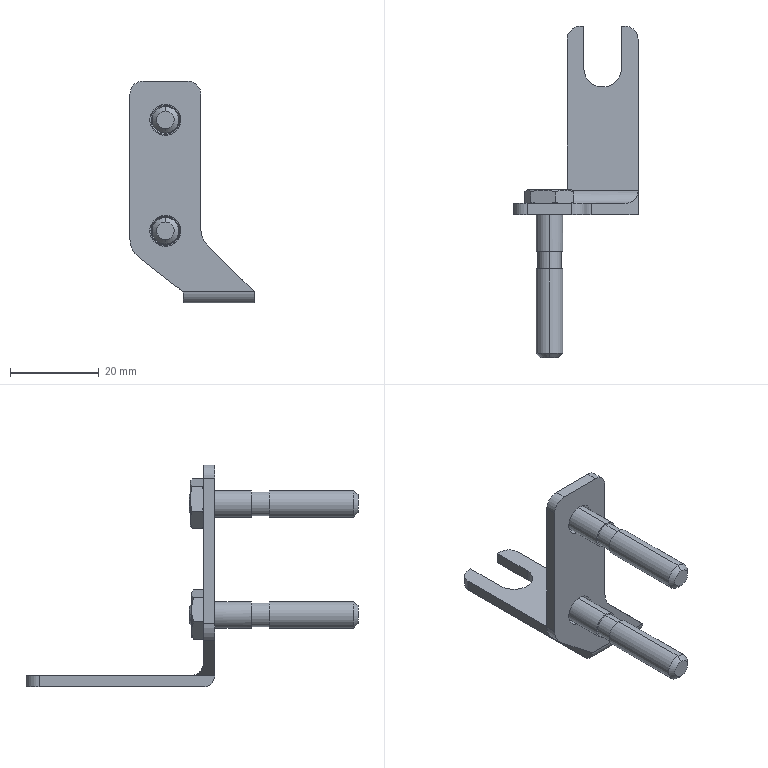Part | SolidWorks | features BaseBody 1 | 1 solid | 115 faces | box 28 x 74.8 x 50 mm | volume 5560 mm3 | plane 43 | cone 39 | cylinder 33 | commonest cylinder face diameters 6 x15 6.5 x6 5.3 x4 7 x4 10 x2 5 x1